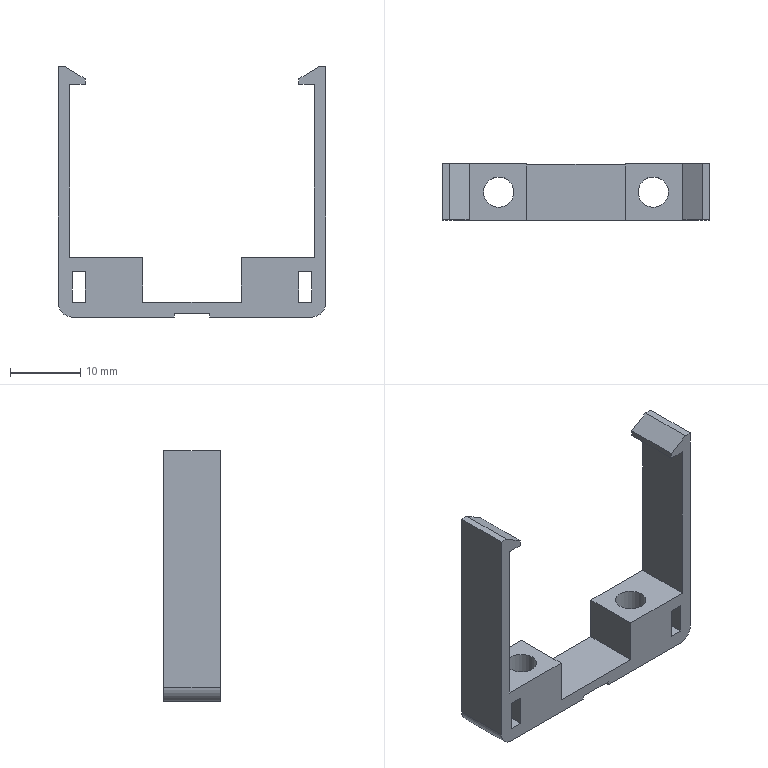Part | NX | 1 solid | 36 faces | box 38 x 8 x 35.6 mm | volume 2200 mm3 | plane 32 | cylinder 4 | commonest cylinder face diameters 4 x2 4.3 x2
STEP:
#1=CARTESIAN_POINT('',(19.85,0.,0.));
#2=VERTEX_POINT('',#1);
#3=CARTESIAN_POINT('',(22.,0.,0.));
#4=DIRECTION('',(0.,0.,1.));
#5=DIRECTION('',(-1.,0.,0.));
#6=AXIS2_PLACEMENT_3D('',#3,#4,#5);
#7=CIRCLE('',#6,2.15);
#8=EDGE_CURVE('',#2,#2,#7,.T.);
#9=ORIENTED_EDGE('',*,*,#8,.T.);
#10=EDGE_LOOP('',(#9));
#11=FACE_BOUND('',#10,.T.);
#12=CARTESIAN_POINT('',(28.,4.,0.));
#13=VERTEX_POINT('',#12);
#14=CARTESIAN_POINT('',(13.5,4.,0.));
#15=VERTEX_POINT('',#14);
#16=CARTESIAN_POINT('',(-8.,4.,0.));
#17=DIRECTION('',(-1.,0.,0.));
#18=VECTOR('',#17,1000.);
#19=LINE('',#16,#18);
#20=EDGE_CURVE('',#13,#15,#19,.T.);
#21=ORIENTED_EDGE('',*,*,#20,.F.);
#22=CARTESIAN_POINT('',(28.,-4.,0.));
#23=VERTEX_POINT('',#22);
#24=CARTESIAN_POINT('',(28.,-4.,0.));
#25=DIRECTION('',(0.,1.,0.));
#26=VECTOR('',#25,1000.);
#27=LINE('',#24,#26);
#28=EDGE_CURVE('',#13,#23,#27,.F.);
#29=ORIENTED_EDGE('',*,*,#28,.T.);
#30=CARTESIAN_POINT('',(13.5,-4.,0.));
#31=VERTEX_POINT('',#30);
#32=CARTESIAN_POINT('',(-8.,-4.,0.));
#33=DIRECTION('',(1.,0.,0.));
#34=VECTOR('',#33,1000.);
#35=LINE('',#32,#34);
#36=EDGE_CURVE('',#31,#23,#35,.T.);
#37=ORIENTED_EDGE('',*,*,#36,.F.);
#38=CARTESIAN_POINT('',(13.5,4.,0.));
#39=DIRECTION('',(0.,-1.,0.));
#40=VECTOR('',#39,1000.);
#41=LINE('',#38,#40);
#42=EDGE_CURVE('',#15,#31,#41,.T.);
#43=ORIENTED_EDGE('',*,*,#42,.F.);
#44=EDGE_LOOP('',(#21,#29,#37,#43));
#45=FACE_BOUND('',#44,.T.);
#46=CARTESIAN_POINT('',(-8.,-4.,0.));
#47=DIRECTION('',(0.,0.,1.));
#48=DIRECTION('',(1.,0.,0.));
#49=AXIS2_PLACEMENT_3D('',#46,#47,#48);
#50=PLANE('',#49);
#51=ADVANCED_FACE('',(#11,#45),#50,.F.);
#52=CARTESIAN_POINT('',(-6.4,-4.,8.5));
#53=VERTEX_POINT('',#52);
#54=CARTESIAN_POINT('',(-6.4,4.,8.5));
#55=VERTEX_POINT('',#54);
#56=CARTESIAN_POINT('',(-6.4,-31.365,8.5));
#57=DIRECTION('',(0.,1.,0.));
#58=VECTOR('',#57,1000.);
#59=LINE('',#56,#58);
#60=EDGE_CURVE('',#53,#55,#59,.T.);
#61=ORIENTED_EDGE('',*,*,#60,.F.);
#62=CARTESIAN_POINT('',(4.,-4.,8.5));
#63=VERTEX_POINT('',#62);
#64=CARTESIAN_POINT('',(-8.,-4.,8.5));
#65=DIRECTION('',(1.,0.,0.));
#66=VECTOR('',#65,1000.);
#67=LINE('',#64,#66);
#68=EDGE_CURVE('',#53,#63,#67,.T.);
#69=ORIENTED_EDGE('',*,*,#68,.T.);
#70=CARTESIAN_POINT('',(4.,4.,8.5));
#71=VERTEX_POINT('',#70);
#72=CARTESIAN_POINT('',(4.,4.,8.5));
#73=DIRECTION('',(0.,-1.,0.));
#74=VECTOR('',#73,1000.);
#75=LINE('',#72,#74);
#76=EDGE_CURVE('',#71,#63,#75,.T.);
#77=ORIENTED_EDGE('',*,*,#76,.F.);
#78=CARTESIAN_POINT('',(-8.,4.,8.5));
#79=DIRECTION('',(-1.,0.,0.));
#80=VECTOR('',#79,1000.);
#81=LINE('',#78,#80);
#82=EDGE_CURVE('',#71,#55,#81,.T.);
#83=ORIENTED_EDGE('',*,*,#82,.T.);
#84=EDGE_LOOP('',(#61,#69,#77,#83));
#85=FACE_BOUND('',#84,.T.);
#86=CARTESIAN_POINT('',(2.15,0.,8.5));
#87=VERTEX_POINT('',#86);
#88=CARTESIAN_POINT('',(0.,0.,8.5));
#89=DIRECTION('',(0.,0.,1.));
#90=DIRECTION('',(1.,0.,0.));
#91=AXIS2_PLACEMENT_3D('',#88,#89,#90);
#92=CIRCLE('',#91,2.15);
#93=EDGE_CURVE('',#87,#87,#92,.T.);
#94=ORIENTED_EDGE('',*,*,#93,.F.);
#95=EDGE_LOOP('',(#94));
#96=FACE_BOUND('',#95,.T.);
#97=CARTESIAN_POINT('',(-8.,-4.,8.5));
#98=DIRECTION('',(0.,0.,1.));
#99=DIRECTION('',(1.,0.,0.));
#100=AXIS2_PLACEMENT_3D('',#97,#98,#99);
#101=PLANE('',#100);
#102=ADVANCED_FACE('',(#85,#96),#101,.T.);
#103=CARTESIAN_POINT('',(28.4,-4.,8.5));
#104=VERTEX_POINT('',#103);
#105=CARTESIAN_POINT('',(28.4,4.,8.5));
#106=VERTEX_POINT('',#105);
#107=CARTESIAN_POINT('',(28.4,-31.365,8.5));
#108=DIRECTION('',(0.,1.,0.));
#109=VECTOR('',#108,1000.);
#110=LINE('',#107,#109);
#111=EDGE_CURVE('',#104,#106,#110,.T.);
#112=ORIENTED_EDGE('',*,*,#111,.T.);
#113=CARTESIAN_POINT('',(18.,4.,8.5));
#114=VERTEX_POINT('',#113);
#115=CARTESIAN_POINT('',(-8.,4.,8.5));
#116=DIRECTION('',(-1.,0.,0.));
#117=VECTOR('',#116,1000.);
#118=LINE('',#115,#117);
#119=EDGE_CURVE('',#106,#114,#118,.T.);
#120=ORIENTED_EDGE('',*,*,#119,.T.);
#121=CARTESIAN_POINT('',(18.,-4.,8.5));
#122=VERTEX_POINT('',#121);
#123=CARTESIAN_POINT('',(18.,4.,8.5));
#124=DIRECTION('',(0.,1.,0.));
#125=VECTOR('',#124,1000.);
#126=LINE('',#123,#125);
#127=EDGE_CURVE('',#122,#114,#126,.T.);
#128=ORIENTED_EDGE('',*,*,#127,.F.);
#129=CARTESIAN_POINT('',(-8.,-4.,8.5));
#130=DIRECTION('',(1.,0.,0.));
#131=VECTOR('',#130,1000.);
#132=LINE('',#129,#131);
#133=EDGE_CURVE('',#122,#104,#132,.T.);
#134=ORIENTED_EDGE('',*,*,#133,.T.);
#135=EDGE_LOOP('',(#112,#120,#128,#134));
#136=FACE_BOUND('',#135,.T.);
#137=CARTESIAN_POINT('',(19.85,0.,8.5));
#138=VERTEX_POINT('',#137);
#139=CARTESIAN_POINT('',(22.,0.,8.5));
#140=DIRECTION('',(0.,0.,1.));
#141=DIRECTION('',(-1.,0.,0.));
#142=AXIS2_PLACEMENT_3D('',#139,#140,#141);
#143=CIRCLE('',#142,2.15);
#144=EDGE_CURVE('',#138,#138,#143,.T.);
#145=ORIENTED_EDGE('',*,*,#144,.F.);
#146=EDGE_LOOP('',(#145));
#147=FACE_BOUND('',#146,.T.);
#148=CARTESIAN_POINT('',(-8.,-4.,8.5));
#149=DIRECTION('',(0.,0.,1.));
#150=DIRECTION('',(1.,0.,0.));
#151=AXIS2_PLACEMENT_3D('',#148,#149,#150);
#152=PLANE('',#151);
#153=ADVANCED_FACE('',(#136,#147),#152,.T.);
#154=CARTESIAN_POINT('',(2.15,0.,0.));
#155=VERTEX_POINT('',#154);
#156=CARTESIAN_POINT('',(0.,0.,0.));
#157=DIRECTION('',(0.,0.,1.));
#158=DIRECTION('',(1.,0.,0.));
#159=AXIS2_PLACEMENT_3D('',#156,#157,#158);
#160=CIRCLE('',#159,2.15);
#161=EDGE_CURVE('',#155,#155,#160,.T.);
#162=ORIENTED_EDGE('',*,*,#161,.T.);
#163=EDGE_LOOP('',(#162));
#164=FACE_BOUND('',#163,.T.);
#165=CARTESIAN_POINT('',(-6.,-4.,0.));
#166=VERTEX_POINT('',#165);
#167=CARTESIAN_POINT('',(8.5,-4.,0.));
#168=VERTEX_POINT('',#167);
#169=CARTESIAN_POINT('',(-8.,-4.,0.));
#170=DIRECTION('',(1.,0.,0.));
#171=VECTOR('',#170,1000.);
#172=LINE('',#169,#171);
#173=EDGE_CURVE('',#166,#168,#172,.T.);
#174=ORIENTED_EDGE('',*,*,#173,.F.);
#175=CARTESIAN_POINT('',(-6.,4.,0.));
#176=VERTEX_POINT('',#175);
#177=CARTESIAN_POINT('',(-6.,-4.,0.));
#178=DIRECTION('',(0.,-1.,0.));
#179=VECTOR('',#178,1000.);
#180=LINE('',#177,#179);
#181=EDGE_CURVE('',#166,#176,#180,.F.);
#182=ORIENTED_EDGE('',*,*,#181,.T.);
#183=CARTESIAN_POINT('',(8.5,4.,0.));
#184=VERTEX_POINT('',#183);
#185=CARTESIAN_POINT('',(-8.,4.,0.));
#186=DIRECTION('',(-1.,0.,0.));
#187=VECTOR('',#186,1000.);
#188=LINE('',#185,#187);
#189=EDGE_CURVE('',#184,#176,#188,.T.);
#190=ORIENTED_EDGE('',*,*,#189,.F.);
#191=CARTESIAN_POINT('',(8.5,4.,0.));
#192=DIRECTION('',(0.,1.,0.));
#193=VECTOR('',#192,1000.);
#194=LINE('',#191,#193);
#195=EDGE_CURVE('',#168,#184,#194,.T.);
#196=ORIENTED_EDGE('',*,*,#195,.F.);
#197=EDGE_LOOP('',(#174,#182,#190,#196));
#198=FACE_BOUND('',#197,.T.);
#199=CARTESIAN_POINT('',(-8.,-4.,0.));
#200=DIRECTION('',(0.,0.,1.));
#201=DIRECTION('',(1.,0.,0.));
#202=AXIS2_PLACEMENT_3D('',#199,#200,#201);
#203=PLANE('',#202);
#204=ADVANCED_FACE('',(#164,#198),#203,.F.);
#205=CARTESIAN_POINT('',(-8.,4.,35.6));
#206=VERTEX_POINT('',#205);
#207=CARTESIAN_POINT('',(-8.,4.,2.));
#208=VERTEX_POINT('',#207);
#209=CARTESIAN_POINT('',(-8.,4.,8.5));
#210=DIRECTION('',(0.,0.,-1.));
#211=VECTOR('',#210,1000.);
#212=LINE('',#209,#211);
#213=EDGE_CURVE('',#206,#208,#212,.T.);
#214=ORIENTED_EDGE('',*,*,#213,.T.);
#215=CARTESIAN_POINT('',(-8.,-4.,2.));
#216=VERTEX_POINT('',#215);
#217=CARTESIAN_POINT('',(-8.,4.,2.));
#218=DIRECTION('',(0.,-1.,0.));
#219=VECTOR('',#218,1000.);
#220=LINE('',#217,#219);
#221=EDGE_CURVE('',#208,#216,#220,.T.);
#222=ORIENTED_EDGE('',*,*,#221,.T.);
#223=CARTESIAN_POINT('',(-8.,-4.,35.6));
#224=VERTEX_POINT('',#223);
#225=CARTESIAN_POINT('',(-8.,-4.,8.5));
#226=DIRECTION('',(0.,0.,-1.));
#227=VECTOR('',#226,1000.);
#228=LINE('',#225,#227);
#229=EDGE_CURVE('',#224,#216,#228,.T.);
#230=ORIENTED_EDGE('',*,*,#229,.F.);
#231=CARTESIAN_POINT('',(-8.,-31.365,35.6));
#232=DIRECTION('',(0.,1.,0.));
#233=VECTOR('',#232,1000.);
#234=LINE('',#231,#233);
#235=EDGE_CURVE('',#224,#206,#234,.T.);
#236=ORIENTED_EDGE('',*,*,#235,.T.);
#237=EDGE_LOOP('',(#214,#222,#230,#236));
#238=FACE_BOUND('',#237,.T.);
#239=CARTESIAN_POINT('',(-8.,4.,8.5));
#240=DIRECTION('',(1.,0.,0.));
#241=DIRECTION('',(0.,0.,-1.));
#242=AXIS2_PLACEMENT_3D('',#239,#240,#241);
#243=PLANE('',#242);
#244=ADVANCED_FACE('',(#238),#243,.F.);
#245=CARTESIAN_POINT('',(28.,-4.,6.5));
#246=VERTEX_POINT('',#245);
#247=CARTESIAN_POINT('',(28.,-4.,2.1));
#248=VERTEX_POINT('',#247);
#249=CARTESIAN_POINT('',(28.,-4.,2.1));
#250=DIRECTION('',(0.,0.,-1.));
#251=VECTOR('',#250,1000.);
#252=LINE('',#249,#251);
#253=EDGE_CURVE('',#246,#248,#252,.T.);
#254=ORIENTED_EDGE('',*,*,#253,.T.);
#255=CARTESIAN_POINT('',(26.15,-4.,2.1));
#256=VERTEX_POINT('',#255);
#257=CARTESIAN_POINT('',(28.,-4.,2.1));
#258=DIRECTION('',(-1.,0.,0.));
#259=VECTOR('',#258,1000.);
#260=LINE('',#257,#259);
#261=EDGE_CURVE('',#248,#256,#260,.T.);
#262=ORIENTED_EDGE('',*,*,#261,.T.);
#263=CARTESIAN_POINT('',(26.15,-4.,6.5));
#264=VERTEX_POINT('',#263);
#265=CARTESIAN_POINT('',(26.15,-4.,2.1));
#266=DIRECTION('',(0.,0.,1.));
#267=VECTOR('',#266,1000.);
#268=LINE('',#265,#267);
#269=EDGE_CURVE('',#256,#264,#268,.T.);
#270=ORIENTED_EDGE('',*,*,#269,.T.);
#271=CARTESIAN_POINT('',(28.,-4.,6.5));
#272=DIRECTION('',(1.,0.,0.));
#273=VECTOR('',#272,1000.);
#274=LINE('',#271,#273);
#275=EDGE_CURVE('',#264,#246,#274,.T.);
#276=ORIENTED_EDGE('',*,*,#275,.T.);
#277=EDGE_LOOP('',(#254,#262,#270,#276));
#278=FACE_BOUND('',#277,.T.);
#279=CARTESIAN_POINT('',(-4.15,-4.,2.1));
#280=VERTEX_POINT('',#279);
#281=CARTESIAN_POINT('',(-6.,-4.,2.1));
#282=VERTEX_POINT('',#281);
#283=CARTESIAN_POINT('',(-6.,-4.,2.1));
#284=DIRECTION('',(-1.,0.,0.));
#285=VECTOR('',#284,1000.);
#286=LINE('',#283,#285);
#287=EDGE_CURVE('',#280,#282,#286,.T.);
#288=ORIENTED_EDGE('',*,*,#287,.T.);
#289=CARTESIAN_POINT('',(-6.,-4.,6.5));
#290=VERTEX_POINT('',#289);
#291=CARTESIAN_POINT('',(-6.,-4.,2.1));
#292=DIRECTION('',(0.,0.,1.));
#293=VECTOR('',#292,1000.);
#294=LINE('',#291,#293);
#295=EDGE_CURVE('',#282,#290,#294,.T.);
#296=ORIENTED_EDGE('',*,*,#295,.T.);
#297=CARTESIAN_POINT('',(-4.15,-4.,6.5));
#298=VERTEX_POINT('',#297);
#299=CARTESIAN_POINT('',(-6.,-4.,6.5));
#300=DIRECTION('',(1.,0.,0.));
#301=VECTOR('',#300,1000.);
#302=LINE('',#299,#301);
#303=EDGE_CURVE('',#290,#298,#302,.T.);
#304=ORIENTED_EDGE('',*,*,#303,.T.);
#305=CARTESIAN_POINT('',(-4.15,-4.,2.1));
#306=DIRECTION('',(0.,0.,-1.));
#307=VECTOR('',#306,1000.);
#308=LINE('',#305,#307);
#309=EDGE_CURVE('',#298,#280,#308,.T.);
#310=ORIENTED_EDGE('',*,*,#309,.T.);
#311=EDGE_LOOP('',(#288,#296,#304,#310));
#312=FACE_BOUND('',#311,.T.);
#313=ORIENTED_EDGE('',*,*,#229,.T.);
#314=CARTESIAN_POINT('',(-6.,-4.,2.));
#315=DIRECTION('',(0.,1.,0.));
#316=DIRECTION('',(-1.,0.,0.));
#317=AXIS2_PLACEMENT_3D('',#314,#315,#316);
#318=CIRCLE('',#317,2.);
#319=EDGE_CURVE('',#216,#166,#318,.F.);
#320=ORIENTED_EDGE('',*,*,#319,.T.);
#321=ORIENTED_EDGE('',*,*,#173,.T.);
#322=CARTESIAN_POINT('',(8.5,-4.,0.5));
#323=VERTEX_POINT('',#322);
#324=CARTESIAN_POINT('',(8.5,-4.,0.5));
#325=DIRECTION('',(0.,0.,-1.));
#326=VECTOR('',#325,1000.);
#327=LINE('',#324,#326);
#328=EDGE_CURVE('',#323,#168,#327,.T.);
#329=ORIENTED_EDGE('',*,*,#328,.F.);
#330=CARTESIAN_POINT('',(13.5,-4.,0.5));
#331=VERTEX_POINT('',#330);
#332=CARTESIAN_POINT('',(13.5,-4.,0.5));
#333=DIRECTION('',(-1.,0.,0.));
#334=VECTOR('',#333,1000.);
#335=LINE('',#332,#334);
#336=EDGE_CURVE('',#331,#323,#335,.T.);
#337=ORIENTED_EDGE('',*,*,#336,.F.);
#338=CARTESIAN_POINT('',(13.5,-4.,0.5));
#339=DIRECTION('',(0.,0.,-1.));
#340=VECTOR('',#339,1000.);
#341=LINE('',#338,#340);
#342=EDGE_CURVE('',#331,#31,#341,.T.);
#343=ORIENTED_EDGE('',*,*,#342,.T.);
#344=ORIENTED_EDGE('',*,*,#36,.T.);
#345=CARTESIAN_POINT('',(30.,-4.,2.));
#346=VERTEX_POINT('',#345);
#347=CARTESIAN_POINT('',(28.,-4.,2.));
#348=DIRECTION('',(0.,1.,0.));
#349=DIRECTION('',(-1.,0.,0.));
#350=AXIS2_PLACEMENT_3D('',#347,#348,#349);
#351=CIRCLE('',#350,2.);
#352=EDGE_CURVE('',#23,#346,#351,.F.);
#353=ORIENTED_EDGE('',*,*,#352,.T.);
#354=CARTESIAN_POINT('',(30.,-4.,35.6));
#355=VERTEX_POINT('',#354);
#356=CARTESIAN_POINT('',(30.,-4.,8.5));
#357=DIRECTION('',(0.,0.,-1.));
#358=VECTOR('',#357,1000.);
#359=LINE('',#356,#358);
#360=EDGE_CURVE('',#355,#346,#359,.T.);
#361=ORIENTED_EDGE('',*,*,#360,.F.);
#362=CARTESIAN_POINT('',(29.,-4.,35.6));
#363=VERTEX_POINT('',#362);
#364=CARTESIAN_POINT('',(30.,-4.,35.6));
#365=DIRECTION('',(-1.,0.,0.));
#366=VECTOR('',#365,1000.);
#367=LINE('',#364,#366);
#368=EDGE_CURVE('',#355,#363,#367,.T.);
#369=ORIENTED_EDGE('',*,*,#368,.T.);
#370=CARTESIAN_POINT('',(26.2,-4.,33.9));
#371=VERTEX_POINT('',#370);
#372=CARTESIAN_POINT('',(26.2,-4.,33.9));
#373=DIRECTION('',(-0.8548,0.,-0.519));
#374=VECTOR('',#373,1000.);
#375=LINE('',#372,#374);
#376=EDGE_CURVE('',#363,#371,#375,.T.);
#377=ORIENTED_EDGE('',*,*,#376,.T.);
#378=CARTESIAN_POINT('',(26.2,-4.,33.1));
#379=VERTEX_POINT('',#378);
#380=CARTESIAN_POINT('',(26.2,-4.,33.1));
#381=DIRECTION('',(0.,0.,-1.));
#382=VECTOR('',#381,1000.);
#383=LINE('',#380,#382);
#384=EDGE_CURVE('',#371,#379,#383,.T.);
#385=ORIENTED_EDGE('',*,*,#384,.T.);
#386=CARTESIAN_POINT('',(28.4,-4.,33.1));
#387=VERTEX_POINT('',#386);
#388=CARTESIAN_POINT('',(28.4,-4.,33.1));
#389=DIRECTION('',(1.,0.,0.));
#390=VECTOR('',#389,1000.);
#391=LINE('',#388,#390);
#392=EDGE_CURVE('',#379,#387,#391,.T.);
#393=ORIENTED_EDGE('',*,*,#392,.T.);
#394=CARTESIAN_POINT('',(28.4,-4.,8.5));
#395=DIRECTION('',(0.,0.,-1.));
#396=VECTOR('',#395,1000.);
#397=LINE('',#394,#396);
#398=EDGE_CURVE('',#387,#104,#397,.T.);
#399=ORIENTED_EDGE('',*,*,#398,.T.);
#400=ORIENTED_EDGE('',*,*,#133,.F.);
#401=CARTESIAN_POINT('',(18.,-4.,2.1));
#402=VERTEX_POINT('',#401);
#403=CARTESIAN_POINT('',(18.,-4.,-16.125));
#404=DIRECTION('',(0.,0.,1.));
#405=VECTOR('',#404,1000.);
#406=LINE('',#403,#405);
#407=EDGE_CURVE('',#402,#122,#406,.T.);
#408=ORIENTED_EDGE('',*,*,#407,.F.);
#409=CARTESIAN_POINT('',(4.,-4.,2.1));
#410=VERTEX_POINT('',#409);
#411=CARTESIAN_POINT('',(4.,-4.,2.1));
#412=DIRECTION('',(-1.,0.,0.));
#413=VECTOR('',#412,1000.);
#414=LINE('',#411,#413);
#415=EDGE_CURVE('',#402,#410,#414,.T.);
#416=ORIENTED_EDGE('',*,*,#415,.T.);
#417=CARTESIAN_POINT('',(4.,-4.,-16.125));
#418=DIRECTION('',(0.,0.,1.));
#419=VECTOR('',#418,1000.);
#420=LINE('',#417,#419);
#421=EDGE_CURVE('',#410,#63,#420,.T.);
#422=ORIENTED_EDGE('',*,*,#421,.T.);
#423=ORIENTED_EDGE('',*,*,#68,.F.);
#424=CARTESIAN_POINT('',(-6.4,-4.,33.1));
#425=VERTEX_POINT('',#424);
#426=CARTESIAN_POINT('',(-6.4,-4.,8.5));
#427=DIRECTION('',(0.,0.,1.));
#428=VECTOR('',#427,1000.);
#429=LINE('',#426,#428);
#430=EDGE_CURVE('',#53,#425,#429,.T.);
#431=ORIENTED_EDGE('',*,*,#430,.T.);
#432=CARTESIAN_POINT('',(-4.2,-4.,33.1));
#433=VERTEX_POINT('',#432);
#434=CARTESIAN_POINT('',(-6.4,-4.,33.1));
#435=DIRECTION('',(1.,0.,0.));
#436=VECTOR('',#435,1000.);
#437=LINE('',#434,#436);
#438=EDGE_CURVE('',#425,#433,#437,.T.);
#439=ORIENTED_EDGE('',*,*,#438,.T.);
#440=CARTESIAN_POINT('',(-4.2,-4.,33.9));
#441=VERTEX_POINT('',#440);
#442=CARTESIAN_POINT('',(-4.2,-4.,33.1));
#443=DIRECTION('',(0.,0.,1.));
#444=VECTOR('',#443,1000.);
#445=LINE('',#442,#444);
#446=EDGE_CURVE('',#433,#441,#445,.T.);
#447=ORIENTED_EDGE('',*,*,#446,.T.);
#448=CARTESIAN_POINT('',(-7.,-4.,35.6));
#449=VERTEX_POINT('',#448);
#450=CARTESIAN_POINT('',(-4.2,-4.,33.9));
#451=DIRECTION('',(-0.8548,0.,0.519));
#452=VECTOR('',#451,1000.);
#453=LINE('',#450,#452);
#454=EDGE_CURVE('',#441,#449,#453,.T.);
#455=ORIENTED_EDGE('',*,*,#454,.T.);
#456=CARTESIAN_POINT('',(-8.,-4.,35.6));
#457=DIRECTION('',(-1.,0.,0.));
#458=VECTOR('',#457,1000.);
#459=LINE('',#456,#458);
#460=EDGE_CURVE('',#449,#224,#459,.T.);
#461=ORIENTED_EDGE('',*,*,#460,.T.);
#462=EDGE_LOOP('',(#313,#320,#321,#329,#337,#343,#344,#353,#361,#369,#377,#385,#393,#399,#400,#408,#416,#422,#423,#431,#439,#447,#455,#461));
#463=FACE_BOUND('',#462,.T.);
#464=CARTESIAN_POINT('',(-8.,-4.,8.5));
#465=DIRECTION('',(0.,1.,0.));
#466=DIRECTION('',(-1.,0.,0.));
#467=AXIS2_PLACEMENT_3D('',#464,#465,#466);
#468=PLANE('',#467);
#469=ADVANCED_FACE('',(#278,#312,#463),#468,.F.);
#470=ORIENTED_EDGE('',*,*,#360,.T.);
#471=CARTESIAN_POINT('',(30.,4.,2.));
#472=VERTEX_POINT('',#471);
#473=CARTESIAN_POINT('',(30.,4.,2.));
#474=DIRECTION('',(0.,1.,0.));
#475=VECTOR('',#474,1000.);
#476=LINE('',#473,#475);
#477=EDGE_CURVE('',#346,#472,#476,.T.);
#478=ORIENTED_EDGE('',*,*,#477,.T.);
#479=CARTESIAN_POINT('',(30.,4.,35.6));
#480=VERTEX_POINT('',#479);
#481=CARTESIAN_POINT('',(30.,4.,8.5));
#482=DIRECTION('',(0.,0.,-1.));
#483=VECTOR('',#482,1000.);
#484=LINE('',#481,#483);
#485=EDGE_CURVE('',#480,#472,#484,.T.);
#486=ORIENTED_EDGE('',*,*,#485,.F.);
#487=CARTESIAN_POINT('',(30.,-31.365,35.6));
#488=DIRECTION('',(0.,1.,0.));
#489=VECTOR('',#488,1000.);
#490=LINE('',#487,#489);
#491=EDGE_CURVE('',#355,#480,#490,.T.);
#492=ORIENTED_EDGE('',*,*,#491,.F.);
#493=EDGE_LOOP('',(#470,#478,#486,#492));
#494=FACE_BOUND('',#493,.T.);
#495=CARTESIAN_POINT('',(30.,4.,8.5));
#496=DIRECTION('',(-1.,0.,0.));
#497=DIRECTION('',(0.,0.,1.));
#498=AXIS2_PLACEMENT_3D('',#495,#496,#497);
#499=PLANE('',#498);
#500=ADVANCED_FACE('',(#494),#499,.F.);
#501=ORIENTED_EDGE('',*,*,#189,.T.);
#502=CARTESIAN_POINT('',(-6.,4.,2.));
#503=DIRECTION('',(0.,-1.,0.));
#504=DIRECTION('',(1.,0.,0.));
#505=AXIS2_PLACEMENT_3D('',#502,#503,#504);
#506=CIRCLE('',#505,2.);
#507=EDGE_CURVE('',#176,#208,#506,.F.);
#508=ORIENTED_EDGE('',*,*,#507,.T.);
#509=ORIENTED_EDGE('',*,*,#213,.F.);
#510=CARTESIAN_POINT('',(-7.,4.,35.6));
#511=VERTEX_POINT('',#510);
#512=CARTESIAN_POINT('',(-8.,4.,35.6));
#513=DIRECTION('',(1.,0.,0.));
#514=VECTOR('',#513,1000.);
#515=LINE('',#512,#514);
#516=EDGE_CURVE('',#206,#511,#515,.T.);
#517=ORIENTED_EDGE('',*,*,#516,.T.);
#518=CARTESIAN_POINT('',(-4.2,4.,33.9));
#519=VERTEX_POINT('',#518);
#520=CARTESIAN_POINT('',(-4.2,4.,33.9));
#521=DIRECTION('',(0.8548,0.,-0.519));
#522=VECTOR('',#521,1000.);
#523=LINE('',#520,#522);
#524=EDGE_CURVE('',#511,#519,#523,.T.);
#525=ORIENTED_EDGE('',*,*,#524,.T.);
#526=CARTESIAN_POINT('',(-4.2,4.,33.1));
#527=VERTEX_POINT('',#526);
#528=CARTESIAN_POINT('',(-4.2,4.,33.1));
#529=DIRECTION('',(0.,0.,-1.));
#530=VECTOR('',#529,1000.);
#531=LINE('',#528,#530);
#532=EDGE_CURVE('',#519,#527,#531,.T.);
#533=ORIENTED_EDGE('',*,*,#532,.T.);
#534=CARTESIAN_POINT('',(-6.4,4.,33.1));
#535=VERTEX_POINT('',#534);
#536=CARTESIAN_POINT('',(-6.4,4.,33.1));
#537=DIRECTION('',(-1.,0.,0.));
#538=VECTOR('',#537,1000.);
#539=LINE('',#536,#538);
#540=EDGE_CURVE('',#527,#535,#539,.T.);
#541=ORIENTED_EDGE('',*,*,#540,.T.);
#542=CARTESIAN_POINT('',(-6.4,4.,8.5));
#543=DIRECTION('',(0.,0.,-1.));
#544=VECTOR('',#543,1000.);
#545=LINE('',#542,#544);
#546=EDGE_CURVE('',#535,#55,#545,.T.);
#547=ORIENTED_EDGE('',*,*,#546,.T.);
#548=ORIENTED_EDGE('',*,*,#82,.F.);
#549=CARTESIAN_POINT('',(4.,4.,2.1));
#550=VERTEX_POINT('',#549);
#551=CARTESIAN_POINT('',(4.,4.,-16.125));
#552=DIRECTION('',(0.,0.,1.));
#553=VECTOR('',#552,1000.);
#554=LINE('',#551,#553);
#555=EDGE_CURVE('',#550,#71,#554,.T.);
#556=ORIENTED_EDGE('',*,*,#555,.F.);
#557=CARTESIAN_POINT('',(18.,4.,2.1));
#558=VERTEX_POINT('',#557);
#559=CARTESIAN_POINT('',(4.,4.,2.1));
#560=DIRECTION('',(1.,0.,0.));
#561=VECTOR('',#560,1000.);
#562=LINE('',#559,#561);
#563=EDGE_CURVE('',#550,#558,#562,.T.);
#564=ORIENTED_EDGE('',*,*,#563,.T.);
#565=CARTESIAN_POINT('',(18.,4.,-16.125));
#566=DIRECTION('',(0.,0.,1.));
#567=VECTOR('',#566,1000.);
#568=LINE('',#565,#567);
#569=EDGE_CURVE('',#558,#114,#568,.T.);
#570=ORIENTED_EDGE('',*,*,#569,.T.);
#571=ORIENTED_EDGE('',*,*,#119,.F.);
#572=CARTESIAN_POINT('',(28.4,4.,33.1));
#573=VERTEX_POINT('',#572);
#574=CARTESIAN_POINT('',(28.4,4.,8.5));
#575=DIRECTION('',(0.,0.,1.));
#576=VECTOR('',#575,1000.);
#577=LINE('',#574,#576);
#578=EDGE_CURVE('',#106,#573,#577,.T.);
#579=ORIENTED_EDGE('',*,*,#578,.T.);
#580=CARTESIAN_POINT('',(26.2,4.,33.1));
#581=VERTEX_POINT('',#580);
#582=CARTESIAN_POINT('',(28.4,4.,33.1));
#583=DIRECTION('',(-1.,0.,0.));
#584=VECTOR('',#583,1000.);
#585=LINE('',#582,#584);
#586=EDGE_CURVE('',#573,#581,#585,.T.);
#587=ORIENTED_EDGE('',*,*,#586,.T.);
#588=CARTESIAN_POINT('',(26.2,4.,33.9));
#589=VERTEX_POINT('',#588);
#590=CARTESIAN_POINT('',(26.2,4.,33.1));
#591=DIRECTION('',(0.,0.,1.));
#592=VECTOR('',#591,1000.);
#593=LINE('',#590,#592);
#594=EDGE_CURVE('',#581,#589,#593,.T.);
#595=ORIENTED_EDGE('',*,*,#594,.T.);
#596=CARTESIAN_POINT('',(29.,4.,35.6));
#597=VERTEX_POINT('',#596);
#598=CARTESIAN_POINT('',(26.2,4.,33.9));
#599=DIRECTION('',(0.8548,0.,0.519));
#600=VECTOR('',#599,1000.);
#601=LINE('',#598,#600);
#602=EDGE_CURVE('',#589,#597,#601,.T.);
#603=ORIENTED_EDGE('',*,*,#602,.T.);
#604=CARTESIAN_POINT('',(30.,4.,35.6));
#605=DIRECTION('',(1.,0.,0.));
#606=VECTOR('',#605,1000.);
#607=LINE('',#604,#606);
#608=EDGE_CURVE('',#597,#480,#607,.T.);
#609=ORIENTED_EDGE('',*,*,#608,.T.);
#610=ORIENTED_EDGE('',*,*,#485,.T.);
#611=CARTESIAN_POINT('',(28.,4.,2.));
#612=DIRECTION('',(0.,-1.,0.));
#613=DIRECTION('',(1.,0.,0.));
#614=AXIS2_PLACEMENT_3D('',#611,#612,#613);
#615=CIRCLE('',#614,2.);
#616=EDGE_CURVE('',#472,#13,#615,.F.);
#617=ORIENTED_EDGE('',*,*,#616,.T.);
#618=ORIENTED_EDGE('',*,*,#20,.T.);
#619=CARTESIAN_POINT('',(13.5,4.,0.5));
#620=VERTEX_POINT('',#619);
#621=CARTESIAN_POINT('',(13.5,4.,0.5));
#622=DIRECTION('',(0.,0.,-1.));
#623=VECTOR('',#622,1000.);
#624=LINE('',#621,#623);
#625=EDGE_CURVE('',#620,#15,#624,.T.);
#626=ORIENTED_EDGE('',*,*,#625,.F.);
#627=CARTESIAN_POINT('',(8.5,4.,0.5));
#628=VERTEX_POINT('',#627);
#629=CARTESIAN_POINT('',(13.5,4.,0.5));
#630=DIRECTION('',(1.,0.,0.));
#631=VECTOR('',#630,1000.);
#632=LINE('',#629,#631);
#633=EDGE_CURVE('',#628,#620,#632,.T.);
#634=ORIENTED_EDGE('',*,*,#633,.F.);
#635=CARTESIAN_POINT('',(8.5,4.,0.5));
#636=DIRECTION('',(0.,0.,-1.));
#637=VECTOR('',#636,1000.);
#638=LINE('',#635,#637);
#639=EDGE_CURVE('',#628,#184,#638,.T.);
#640=ORIENTED_EDGE('',*,*,#639,.T.);
#641=EDGE_LOOP('',(#501,#508,#509,#517,#525,#533,#541,#547,#548,#556,#564,#570,#571,#579,#587,#595,#603,#609,#610,#617,#618,#626,#634,#640));
#642=FACE_BOUND('',#641,.T.);
#643=CARTESIAN_POINT('',(26.15,4.,2.1));
#644=VERTEX_POINT('',#643);
#645=CARTESIAN_POINT('',(26.15,4.,6.5));
#646=VERTEX_POINT('',#645);
#647=CARTESIAN_POINT('',(26.15,4.,2.1));
#648=DIRECTION('',(0.,0.,1.));
#649=VECTOR('',#648,1000.);
#650=LINE('',#647,#649);
#651=EDGE_CURVE('',#644,#646,#650,.T.);
#652=ORIENTED_EDGE('',*,*,#651,.F.);
#653=CARTESIAN_POINT('',(28.,4.,2.1));
#654=VERTEX_POINT('',#653);
#655=CARTESIAN_POINT('',(28.,4.,2.1));
#656=DIRECTION('',(-1.,0.,0.));
#657=VECTOR('',#656,1000.);
#658=LINE('',#655,#657);
#659=EDGE_CURVE('',#654,#644,#658,.T.);
#660=ORIENTED_EDGE('',*,*,#659,.F.);
#661=CARTESIAN_POINT('',(28.,4.,6.5));
#662=VERTEX_POINT('',#661);
#663=CARTESIAN_POINT('',(28.,4.,2.1));
#664=DIRECTION('',(0.,0.,-1.));
#665=VECTOR('',#664,1000.);
#666=LINE('',#663,#665);
#667=EDGE_CURVE('',#662,#654,#666,.T.);
#668=ORIENTED_EDGE('',*,*,#667,.F.);
#669=CARTESIAN_POINT('',(28.,4.,6.5));
#670=DIRECTION('',(1.,0.,0.));
#671=VECTOR('',#670,1000.);
#672=LINE('',#669,#671);
#673=EDGE_CURVE('',#646,#662,#672,.T.);
#674=ORIENTED_EDGE('',*,*,#673,.F.);
#675=EDGE_LOOP('',(#652,#660,#668,#674));
#676=FACE_BOUND('',#675,.T.);
#677=CARTESIAN_POINT('',(-6.,4.,6.5));
#678=VERTEX_POINT('',#677);
#679=CARTESIAN_POINT('',(-4.15,4.,6.5));
#680=VERTEX_POINT('',#679);
#681=CARTESIAN_POINT('',(-6.,4.,6.5));
#682=DIRECTION('',(1.,0.,0.));
#683=VECTOR('',#682,1000.);
#684=LINE('',#681,#683);
#685=EDGE_CURVE('',#678,#680,#684,.T.);
#686=ORIENTED_EDGE('',*,*,#685,.F.);
#687=CARTESIAN_POINT('',(-6.,4.,2.1));
#688=VERTEX_POINT('',#687);
#689=CARTESIAN_POINT('',(-6.,4.,2.1));
#690=DIRECTION('',(0.,0.,1.));
#691=VECTOR('',#690,1000.);
#692=LINE('',#689,#691);
#693=EDGE_CURVE('',#688,#678,#692,.T.);
#694=ORIENTED_EDGE('',*,*,#693,.F.);
#695=CARTESIAN_POINT('',(-4.15,4.,2.1));
#696=VERTEX_POINT('',#695);
#697=CARTESIAN_POINT('',(-6.,4.,2.1));
#698=DIRECTION('',(-1.,0.,0.));
#699=VECTOR('',#698,1000.);
#700=LINE('',#697,#699);
#701=EDGE_CURVE('',#696,#688,#700,.T.);
#702=ORIENTED_EDGE('',*,*,#701,.F.);
#703=CARTESIAN_POINT('',(-4.15,4.,2.1));
#704=DIRECTION('',(0.,0.,-1.));
#705=VECTOR('',#704,1000.);
#706=LINE('',#703,#705);
#707=EDGE_CURVE('',#680,#696,#706,.T.);
#708=ORIENTED_EDGE('',*,*,#707,.F.);
#709=EDGE_LOOP('',(#686,#694,#702,#708));
#710=FACE_BOUND('',#709,.T.);
#711=CARTESIAN_POINT('',(-8.,4.,8.5));
#712=DIRECTION('',(0.,-1.,0.));
#713=DIRECTION('',(1.,0.,0.));
#714=AXIS2_PLACEMENT_3D('',#711,#712,#713);
#715=PLANE('',#714);
#716=ADVANCED_FACE('',(#642,#676,#710),#715,.F.);
#717=ORIENTED_EDGE('',*,*,#93,.T.);
#718=EDGE_LOOP('',(#717));
#719=FACE_BOUND('',#718,.T.);
#720=ORIENTED_EDGE('',*,*,#161,.F.);
#721=EDGE_LOOP('',(#720));
#722=FACE_BOUND('',#721,.T.);
#723=CARTESIAN_POINT('',(0.,0.,8.5));
#724=DIRECTION('',(0.,0.,-1.));
#725=DIRECTION('',(-1.,0.,0.));
#726=AXIS2_PLACEMENT_3D('',#723,#724,#725);
#727=CYLINDRICAL_SURFACE('',#726,2.15);
#728=ADVANCED_FACE('',(#719,#722),#727,.F.);
#729=ORIENTED_EDGE('',*,*,#144,.T.);
#730=EDGE_LOOP('',(#729));
#731=FACE_BOUND('',#730,.T.);
#732=ORIENTED_EDGE('',*,*,#8,.F.);
#733=EDGE_LOOP('',(#732));
#734=FACE_BOUND('',#733,.T.);
#735=CARTESIAN_POINT('',(22.,0.,8.5));
#736=DIRECTION('',(0.,0.,-1.));
#737=DIRECTION('',(-1.,0.,0.));
#738=AXIS2_PLACEMENT_3D('',#735,#736,#737);
#739=CYLINDRICAL_SURFACE('',#738,2.15);
#740=ADVANCED_FACE('',(#731,#734),#739,.F.);
#741=CARTESIAN_POINT('',(4.,4.,2.1));
#742=DIRECTION('',(0.,1.,0.));
#743=VECTOR('',#742,1000.);
#744=LINE('',#741,#743);
#745=EDGE_CURVE('',#410,#550,#744,.T.);
#746=ORIENTED_EDGE('',*,*,#745,.T.);
#747=ORIENTED_EDGE('',*,*,#555,.T.);
#748=ORIENTED_EDGE('',*,*,#76,.T.);
#749=ORIENTED_EDGE('',*,*,#421,.F.);
#750=EDGE_LOOP('',(#746,#747,#748,#749));
#751=FACE_BOUND('',#750,.T.);
#752=CARTESIAN_POINT('',(4.,4.,-16.125));
#753=DIRECTION('',(-1.,0.,0.));
#754=DIRECTION('',(0.,-1.,0.));
#755=AXIS2_PLACEMENT_3D('',#752,#753,#754);
#756=PLANE('',#755);
#757=ADVANCED_FACE('',(#751),#756,.F.);
#758=CARTESIAN_POINT('',(18.,4.,2.1));
#759=DIRECTION('',(0.,-1.,0.));
#760=VECTOR('',#759,1000.);
#761=LINE('',#758,#760);
#762=EDGE_CURVE('',#558,#402,#761,.T.);
#763=ORIENTED_EDGE('',*,*,#762,.T.);
#764=ORIENTED_EDGE('',*,*,#407,.T.);
#765=ORIENTED_EDGE('',*,*,#127,.T.);
#766=ORIENTED_EDGE('',*,*,#569,.F.);
#767=EDGE_LOOP('',(#763,#764,#765,#766));
#768=FACE_BOUND('',#767,.T.);
#769=CARTESIAN_POINT('',(18.,4.,-16.125));
#770=DIRECTION('',(1.,0.,0.));
#771=DIRECTION('',(0.,0.,-1.));
#772=AXIS2_PLACEMENT_3D('',#769,#770,#771);
#773=PLANE('',#772);
#774=ADVANCED_FACE('',(#768),#773,.F.);
#775=ORIENTED_EDGE('',*,*,#745,.F.);
#776=ORIENTED_EDGE('',*,*,#415,.F.);
#777=ORIENTED_EDGE('',*,*,#762,.F.);
#778=ORIENTED_EDGE('',*,*,#563,.F.);
#779=EDGE_LOOP('',(#775,#776,#777,#778));
#780=FACE_BOUND('',#779,.T.);
#781=CARTESIAN_POINT('',(-8.,-4.,2.1));
#782=DIRECTION('',(0.,0.,1.));
#783=DIRECTION('',(1.,0.,0.));
#784=AXIS2_PLACEMENT_3D('',#781,#782,#783);
#785=PLANE('',#784);
#786=ADVANCED_FACE('',(#780),#785,.T.);
#787=ORIENTED_EDGE('',*,*,#430,.F.);
#788=ORIENTED_EDGE('',*,*,#60,.T.);
#789=ORIENTED_EDGE('',*,*,#546,.F.);
#790=CARTESIAN_POINT('',(-6.4,-31.365,33.1));
#791=DIRECTION('',(0.,1.,0.));
#792=VECTOR('',#791,1000.);
#793=LINE('',#790,#792);
#794=EDGE_CURVE('',#425,#535,#793,.T.);
#795=ORIENTED_EDGE('',*,*,#794,.F.);
#796=EDGE_LOOP('',(#787,#788,#789,#795));
#797=FACE_BOUND('',#796,.T.);
#798=CARTESIAN_POINT('',(-6.4,-31.365,8.5));
#799=DIRECTION('',(1.,0.,0.));
#800=DIRECTION('',(0.,1.,0.));
#801=AXIS2_PLACEMENT_3D('',#798,#799,#800);
#802=PLANE('',#801);
#803=ADVANCED_FACE('',(#797),#802,.T.);
#804=ORIENTED_EDGE('',*,*,#438,.F.);
#805=ORIENTED_EDGE('',*,*,#794,.T.);
#806=ORIENTED_EDGE('',*,*,#540,.F.);
#807=CARTESIAN_POINT('',(-4.2,-31.365,33.1));
#808=DIRECTION('',(0.,1.,0.));
#809=VECTOR('',#808,1000.);
#810=LINE('',#807,#809);
#811=EDGE_CURVE('',#433,#527,#810,.T.);
#812=ORIENTED_EDGE('',*,*,#811,.F.);
#813=EDGE_LOOP('',(#804,#805,#806,#812));
#814=FACE_BOUND('',#813,.T.);
#815=CARTESIAN_POINT('',(-6.4,-31.365,33.1));
#816=DIRECTION('',(0.,0.,-1.));
#817=DIRECTION('',(-1.,0.,0.));
#818=AXIS2_PLACEMENT_3D('',#815,#816,#817);
#819=PLANE('',#818);
#820=ADVANCED_FACE('',(#814),#819,.T.);
#821=ORIENTED_EDGE('',*,*,#446,.F.);
#822=ORIENTED_EDGE('',*,*,#811,.T.);
#823=ORIENTED_EDGE('',*,*,#532,.F.);
#824=CARTESIAN_POINT('',(-4.2,-31.365,33.9));
#825=DIRECTION('',(0.,1.,0.));
#826=VECTOR('',#825,1000.);
#827=LINE('',#824,#826);
#828=EDGE_CURVE('',#441,#519,#827,.T.);
#829=ORIENTED_EDGE('',*,*,#828,.F.);
#830=EDGE_LOOP('',(#821,#822,#823,#829));
#831=FACE_BOUND('',#830,.T.);
#832=CARTESIAN_POINT('',(-4.2,-31.365,33.1));
#833=DIRECTION('',(1.,0.,0.));
#834=DIRECTION('',(0.,1.,0.));
#835=AXIS2_PLACEMENT_3D('',#832,#833,#834);
#836=PLANE('',#835);
#837=ADVANCED_FACE('',(#831),#836,.T.);
#838=ORIENTED_EDGE('',*,*,#454,.F.);
#839=ORIENTED_EDGE('',*,*,#828,.T.);
#840=ORIENTED_EDGE('',*,*,#524,.F.);
#841=CARTESIAN_POINT('',(-7.,-31.365,35.6));
#842=DIRECTION('',(0.,1.,0.));
#843=VECTOR('',#842,1000.);
#844=LINE('',#841,#843);
#845=EDGE_CURVE('',#449,#511,#844,.T.);
#846=ORIENTED_EDGE('',*,*,#845,.F.);
#847=EDGE_LOOP('',(#838,#839,#840,#846));
#848=FACE_BOUND('',#847,.T.);
#849=CARTESIAN_POINT('',(-4.2,-31.365,33.9));
#850=DIRECTION('',(0.519,0.,0.8548));
#851=DIRECTION('',(0.8548,0.,-0.519));
#852=AXIS2_PLACEMENT_3D('',#849,#850,#851);
#853=PLANE('',#852);
#854=ADVANCED_FACE('',(#848),#853,.T.);
#855=ORIENTED_EDGE('',*,*,#460,.F.);
#856=ORIENTED_EDGE('',*,*,#845,.T.);
#857=ORIENTED_EDGE('',*,*,#516,.F.);
#858=ORIENTED_EDGE('',*,*,#235,.F.);
#859=EDGE_LOOP('',(#855,#856,#857,#858));
#860=FACE_BOUND('',#859,.T.);
#861=CARTESIAN_POINT('',(-8.,-31.365,35.6));
#862=DIRECTION('',(0.,0.,1.));
#863=DIRECTION('',(1.,0.,0.));
#864=AXIS2_PLACEMENT_3D('',#861,#862,#863);
#865=PLANE('',#864);
#866=ADVANCED_FACE('',(#860),#865,.T.);
#867=ORIENTED_EDGE('',*,*,#384,.F.);
#868=CARTESIAN_POINT('',(26.2,-31.365,33.9));
#869=DIRECTION('',(0.,1.,0.));
#870=VECTOR('',#869,1000.);
#871=LINE('',#868,#870);
#872=EDGE_CURVE('',#371,#589,#871,.T.);
#873=ORIENTED_EDGE('',*,*,#872,.T.);
#874=ORIENTED_EDGE('',*,*,#594,.F.);
#875=CARTESIAN_POINT('',(26.2,-31.365,33.1));
#876=DIRECTION('',(0.,1.,0.));
#877=VECTOR('',#876,1000.);
#878=LINE('',#875,#877);
#879=EDGE_CURVE('',#379,#581,#878,.T.);
#880=ORIENTED_EDGE('',*,*,#879,.F.);
#881=EDGE_LOOP('',(#867,#873,#874,#880));
#882=FACE_BOUND('',#881,.T.);
#883=CARTESIAN_POINT('',(26.2,-31.365,33.1));
#884=DIRECTION('',(-1.,0.,0.));
#885=DIRECTION('',(0.,-1.,0.));
#886=AXIS2_PLACEMENT_3D('',#883,#884,#885);
#887=PLANE('',#886);
#888=ADVANCED_FACE('',(#882),#887,.T.);
#889=ORIENTED_EDGE('',*,*,#392,.F.);
#890=ORIENTED_EDGE('',*,*,#879,.T.);
#891=ORIENTED_EDGE('',*,*,#586,.F.);
#892=CARTESIAN_POINT('',(28.4,-31.365,33.1));
#893=DIRECTION('',(0.,1.,0.));
#894=VECTOR('',#893,1000.);
#895=LINE('',#892,#894);
#896=EDGE_CURVE('',#387,#573,#895,.T.);
#897=ORIENTED_EDGE('',*,*,#896,.F.);
#898=EDGE_LOOP('',(#889,#890,#891,#897));
#899=FACE_BOUND('',#898,.T.);
#900=CARTESIAN_POINT('',(28.4,-31.365,33.1));
#901=DIRECTION('',(0.,0.,-1.));
#902=DIRECTION('',(-1.,0.,0.));
#903=AXIS2_PLACEMENT_3D('',#900,#901,#902);
#904=PLANE('',#903);
#905=ADVANCED_FACE('',(#899),#904,.T.);
#906=ORIENTED_EDGE('',*,*,#398,.F.);
#907=ORIENTED_EDGE('',*,*,#896,.T.);
#908=ORIENTED_EDGE('',*,*,#578,.F.);
#909=ORIENTED_EDGE('',*,*,#111,.F.);
#910=EDGE_LOOP('',(#906,#907,#908,#909));
#911=FACE_BOUND('',#910,.T.);
#912=CARTESIAN_POINT('',(28.4,-31.365,8.5));
#913=DIRECTION('',(-1.,0.,0.));
#914=DIRECTION('',(0.,-1.,0.));
#915=AXIS2_PLACEMENT_3D('',#912,#913,#914);
#916=PLANE('',#915);
#917=ADVANCED_FACE('',(#911),#916,.T.);
#918=ORIENTED_EDGE('',*,*,#368,.F.);
#919=ORIENTED_EDGE('',*,*,#491,.T.);
#920=ORIENTED_EDGE('',*,*,#608,.F.);
#921=CARTESIAN_POINT('',(29.,-31.365,35.6));
#922=DIRECTION('',(0.,1.,0.));
#923=VECTOR('',#922,1000.);
#924=LINE('',#921,#923);
#925=EDGE_CURVE('',#363,#597,#924,.T.);
#926=ORIENTED_EDGE('',*,*,#925,.F.);
#927=EDGE_LOOP('',(#918,#919,#920,#926));
#928=FACE_BOUND('',#927,.T.);
#929=CARTESIAN_POINT('',(30.,-31.365,35.6));
#930=DIRECTION('',(0.,0.,1.));
#931=DIRECTION('',(1.,0.,0.));
#932=AXIS2_PLACEMENT_3D('',#929,#930,#931);
#933=PLANE('',#932);
#934=ADVANCED_FACE('',(#928),#933,.T.);
#935=ORIENTED_EDGE('',*,*,#376,.F.);
#936=ORIENTED_EDGE('',*,*,#925,.T.);
#937=ORIENTED_EDGE('',*,*,#602,.F.);
#938=ORIENTED_EDGE('',*,*,#872,.F.);
#939=EDGE_LOOP('',(#935,#936,#937,#938));
#940=FACE_BOUND('',#939,.T.);
#941=CARTESIAN_POINT('',(26.2,-31.365,33.9));
#942=DIRECTION('',(-0.519,0.,0.8548));
#943=DIRECTION('',(0.8548,0.,0.519));
#944=AXIS2_PLACEMENT_3D('',#941,#942,#943);
#945=PLANE('',#944);
#946=ADVANCED_FACE('',(#940),#945,.T.);
#947=ORIENTED_EDGE('',*,*,#693,.T.);
#948=CARTESIAN_POINT('',(-6.,-4.,6.5));
#949=DIRECTION('',(0.,1.,0.));
#950=VECTOR('',#949,1000.);
#951=LINE('',#948,#950);
#952=EDGE_CURVE('',#290,#678,#951,.T.);
#953=ORIENTED_EDGE('',*,*,#952,.F.);
#954=ORIENTED_EDGE('',*,*,#295,.F.);
#955=CARTESIAN_POINT('',(-6.,-4.,2.1));
#956=DIRECTION('',(0.,1.,0.));
#957=VECTOR('',#956,1000.);
#958=LINE('',#955,#957);
#959=EDGE_CURVE('',#282,#688,#958,.T.);
#960=ORIENTED_EDGE('',*,*,#959,.T.);
#961=EDGE_LOOP('',(#947,#953,#954,#960));
#962=FACE_BOUND('',#961,.T.);
#963=CARTESIAN_POINT('',(-6.,-4.,2.1));
#964=DIRECTION('',(-1.,0.,0.));
#965=DIRECTION('',(0.,-1.,0.));
#966=AXIS2_PLACEMENT_3D('',#963,#964,#965);
#967=PLANE('',#966);
#968=ADVANCED_FACE('',(#962),#967,.F.);
#969=ORIENTED_EDGE('',*,*,#701,.T.);
#970=ORIENTED_EDGE('',*,*,#959,.F.);
#971=ORIENTED_EDGE('',*,*,#287,.F.);
#972=CARTESIAN_POINT('',(-4.15,-4.,2.1));
#973=DIRECTION('',(0.,1.,0.));
#974=VECTOR('',#973,1000.);
#975=LINE('',#972,#974);
#976=EDGE_CURVE('',#280,#696,#975,.T.);
#977=ORIENTED_EDGE('',*,*,#976,.T.);
#978=EDGE_LOOP('',(#969,#970,#971,#977));
#979=FACE_BOUND('',#978,.T.);
#980=CARTESIAN_POINT('',(-6.,-4.,2.1));
#981=DIRECTION('',(0.,0.,-1.));
#982=DIRECTION('',(-1.,0.,0.));
#983=AXIS2_PLACEMENT_3D('',#980,#981,#982);
#984=PLANE('',#983);
#985=ADVANCED_FACE('',(#979),#984,.F.);
#986=ORIENTED_EDGE('',*,*,#707,.T.);
#987=ORIENTED_EDGE('',*,*,#976,.F.);
#988=ORIENTED_EDGE('',*,*,#309,.F.);
#989=CARTESIAN_POINT('',(-4.15,-4.,6.5));
#990=DIRECTION('',(0.,1.,0.));
#991=VECTOR('',#990,1000.);
#992=LINE('',#989,#991);
#993=EDGE_CURVE('',#298,#680,#992,.T.);
#994=ORIENTED_EDGE('',*,*,#993,.T.);
#995=EDGE_LOOP('',(#986,#987,#988,#994));
#996=FACE_BOUND('',#995,.T.);
#997=CARTESIAN_POINT('',(-4.15,-4.,2.1));
#998=DIRECTION('',(1.,0.,0.));
#999=DIRECTION('',(0.,1.,0.));
#1000=AXIS2_PLACEMENT_3D('',#997,#998,#999);
#1001=PLANE('',#1000);
#1002=ADVANCED_FACE('',(#996),#1001,.F.);
#1003=ORIENTED_EDGE('',*,*,#685,.T.);
#1004=ORIENTED_EDGE('',*,*,#993,.F.);
#1005=ORIENTED_EDGE('',*,*,#303,.F.);
#1006=ORIENTED_EDGE('',*,*,#952,.T.);
#1007=EDGE_LOOP('',(#1003,#1004,#1005,#1006));
#1008=FACE_BOUND('',#1007,.T.);
#1009=CARTESIAN_POINT('',(-6.,-4.,6.5));
#1010=DIRECTION('',(0.,0.,1.));
#1011=DIRECTION('',(1.,0.,0.));
#1012=AXIS2_PLACEMENT_3D('',#1009,#1010,#1011);
#1013=PLANE('',#1012);
#1014=ADVANCED_FACE('',(#1008),#1013,.F.);
#1015=ORIENTED_EDGE('',*,*,#659,.T.);
#1016=CARTESIAN_POINT('',(26.15,-4.,2.1));
#1017=DIRECTION('',(0.,1.,0.));
#1018=VECTOR('',#1017,1000.);
#1019=LINE('',#1016,#1018);
#1020=EDGE_CURVE('',#256,#644,#1019,.T.);
#1021=ORIENTED_EDGE('',*,*,#1020,.F.);
#1022=ORIENTED_EDGE('',*,*,#261,.F.);
#1023=CARTESIAN_POINT('',(28.,-4.,2.1));
#1024=DIRECTION('',(0.,1.,0.));
#1025=VECTOR('',#1024,1000.);
#1026=LINE('',#1023,#1025);
#1027=EDGE_CURVE('',#248,#654,#1026,.T.);
#1028=ORIENTED_EDGE('',*,*,#1027,.T.);
#1029=EDGE_LOOP('',(#1015,#1021,#1022,#1028));
#1030=FACE_BOUND('',#1029,.T.);
#1031=CARTESIAN_POINT('',(28.,-4.,2.1));
#1032=DIRECTION('',(0.,0.,-1.));
#1033=DIRECTION('',(-1.,0.,0.));
#1034=AXIS2_PLACEMENT_3D('',#1031,#1032,#1033);
#1035=PLANE('',#1034);
#1036=ADVANCED_FACE('',(#1030),#1035,.F.);
#1037=ORIENTED_EDGE('',*,*,#667,.T.);
#1038=ORIENTED_EDGE('',*,*,#1027,.F.);
#1039=ORIENTED_EDGE('',*,*,#253,.F.);
#1040=CARTESIAN_POINT('',(28.,-4.,6.5));
#1041=DIRECTION('',(0.,1.,0.));
#1042=VECTOR('',#1041,1000.);
#1043=LINE('',#1040,#1042);
#1044=EDGE_CURVE('',#246,#662,#1043,.T.);
#1045=ORIENTED_EDGE('',*,*,#1044,.T.);
#1046=EDGE_LOOP('',(#1037,#1038,#1039,#1045));
#1047=FACE_BOUND('',#1046,.T.);
#1048=CARTESIAN_POINT('',(28.,-4.,2.1));
#1049=DIRECTION('',(1.,0.,0.));
#1050=DIRECTION('',(0.,1.,0.));
#1051=AXIS2_PLACEMENT_3D('',#1048,#1049,#1050);
#1052=PLANE('',#1051);
#1053=ADVANCED_FACE('',(#1047),#1052,.F.);
#1054=ORIENTED_EDGE('',*,*,#673,.T.);
#1055=ORIENTED_EDGE('',*,*,#1044,.F.);
#1056=ORIENTED_EDGE('',*,*,#275,.F.);
#1057=CARTESIAN_POINT('',(26.15,-4.,6.5));
#1058=DIRECTION('',(0.,1.,0.));
#1059=VECTOR('',#1058,1000.);
#1060=LINE('',#1057,#1059);
#1061=EDGE_CURVE('',#264,#646,#1060,.T.);
#1062=ORIENTED_EDGE('',*,*,#1061,.T.);
#1063=EDGE_LOOP('',(#1054,#1055,#1056,#1062));
#1064=FACE_BOUND('',#1063,.T.);
#1065=CARTESIAN_POINT('',(28.,-4.,6.5));
#1066=DIRECTION('',(0.,0.,1.));
#1067=DIRECTION('',(1.,0.,0.));
#1068=AXIS2_PLACEMENT_3D('',#1065,#1066,#1067);
#1069=PLANE('',#1068);
#1070=ADVANCED_FACE('',(#1064),#1069,.F.);
#1071=ORIENTED_EDGE('',*,*,#651,.T.);
#1072=ORIENTED_EDGE('',*,*,#1061,.F.);
#1073=ORIENTED_EDGE('',*,*,#269,.F.);
#1074=ORIENTED_EDGE('',*,*,#1020,.T.);
#1075=EDGE_LOOP('',(#1071,#1072,#1073,#1074));
#1076=FACE_BOUND('',#1075,.T.);
#1077=CARTESIAN_POINT('',(26.15,-4.,2.1));
#1078=DIRECTION('',(-1.,0.,0.));
#1079=DIRECTION('',(0.,-1.,0.));
#1080=AXIS2_PLACEMENT_3D('',#1077,#1078,#1079);
#1081=PLANE('',#1080);
#1082=ADVANCED_FACE('',(#1076),#1081,.F.);
#1083=ORIENTED_EDGE('',*,*,#42,.T.);
#1084=ORIENTED_EDGE('',*,*,#342,.F.);
#1085=CARTESIAN_POINT('',(13.5,4.,0.5));
#1086=DIRECTION('',(0.,-1.,0.));
#1087=VECTOR('',#1086,1000.);
#1088=LINE('',#1085,#1087);
#1089=EDGE_CURVE('',#620,#331,#1088,.T.);
#1090=ORIENTED_EDGE('',*,*,#1089,.F.);
#1091=ORIENTED_EDGE('',*,*,#625,.T.);
#1092=EDGE_LOOP('',(#1083,#1084,#1090,#1091));
#1093=FACE_BOUND('',#1092,.T.);
#1094=CARTESIAN_POINT('',(13.5,4.,0.5));
#1095=DIRECTION('',(1.,0.,0.));
#1096=DIRECTION('',(0.,1.,0.));
#1097=AXIS2_PLACEMENT_3D('',#1094,#1095,#1096);
#1098=PLANE('',#1097);
#1099=ADVANCED_FACE('',(#1093),#1098,.F.);
#1100=ORIENTED_EDGE('',*,*,#195,.T.);
#1101=ORIENTED_EDGE('',*,*,#639,.F.);
#1102=CARTESIAN_POINT('',(8.5,4.,0.5));
#1103=DIRECTION('',(0.,1.,0.));
#1104=VECTOR('',#1103,1000.);
#1105=LINE('',#1102,#1104);
#1106=EDGE_CURVE('',#323,#628,#1105,.T.);
#1107=ORIENTED_EDGE('',*,*,#1106,.F.);
#1108=ORIENTED_EDGE('',*,*,#328,.T.);
#1109=EDGE_LOOP('',(#1100,#1101,#1107,#1108));
#1110=FACE_BOUND('',#1109,.T.);
#1111=CARTESIAN_POINT('',(8.5,4.,0.5));
#1112=DIRECTION('',(-1.,0.,0.));
#1113=DIRECTION('',(0.,0.,1.));
#1114=AXIS2_PLACEMENT_3D('',#1111,#1112,#1113);
#1115=PLANE('',#1114);
#1116=ADVANCED_FACE('',(#1110),#1115,.F.);
#1117=ORIENTED_EDGE('',*,*,#1089,.T.);
#1118=ORIENTED_EDGE('',*,*,#336,.T.);
#1119=ORIENTED_EDGE('',*,*,#1106,.T.);
#1120=ORIENTED_EDGE('',*,*,#633,.T.);
#1121=EDGE_LOOP('',(#1117,#1118,#1119,#1120));
#1122=FACE_BOUND('',#1121,.T.);
#1123=CARTESIAN_POINT('',(13.5,4.,0.5));
#1124=DIRECTION('',(0.,0.,-1.));
#1125=DIRECTION('',(-1.,0.,0.));
#1126=AXIS2_PLACEMENT_3D('',#1123,#1124,#1125);
#1127=PLANE('',#1126);
#1128=ADVANCED_FACE('',(#1122),#1127,.T.);
#1129=ORIENTED_EDGE('',*,*,#507,.F.);
#1130=ORIENTED_EDGE('',*,*,#181,.F.);
#1131=ORIENTED_EDGE('',*,*,#319,.F.);
#1132=ORIENTED_EDGE('',*,*,#221,.F.);
#1133=EDGE_LOOP('',(#1129,#1130,#1131,#1132));
#1134=FACE_BOUND('',#1133,.T.);
#1135=CARTESIAN_POINT('',(-6.,4.,2.));
#1136=DIRECTION('',(0.,-1.,0.));
#1137=DIRECTION('',(0.,0.,-1.));
#1138=AXIS2_PLACEMENT_3D('',#1135,#1136,#1137);
#1139=CYLINDRICAL_SURFACE('',#1138,2.);
#1140=ADVANCED_FACE('',(#1134),#1139,.T.);
#1141=ORIENTED_EDGE('',*,*,#352,.F.);
#1142=ORIENTED_EDGE('',*,*,#28,.F.);
#1143=ORIENTED_EDGE('',*,*,#616,.F.);
#1144=ORIENTED_EDGE('',*,*,#477,.F.);
#1145=EDGE_LOOP('',(#1141,#1142,#1143,#1144));
#1146=FACE_BOUND('',#1145,.T.);
#1147=CARTESIAN_POINT('',(28.,4.,2.));
#1148=DIRECTION('',(0.,1.,0.));
#1149=DIRECTION('',(0.,0.,1.));
#1150=AXIS2_PLACEMENT_3D('',#1147,#1148,#1149);
#1151=CYLINDRICAL_SURFACE('',#1150,2.);
#1152=ADVANCED_FACE('',(#1146),#1151,.T.);
#1153=CLOSED_SHELL('',(#51,#102,#153,#204,#244,#469,#500,#716,#728,#740,#757,#774,#786,#803,#820,#837,#854,#866,#888,#905,#917,#934,#946,#968,#985,#1002,#1014,#1036,#1053,#1070,#1082,#1099,#1116,#1128,#1140,#1152));
#1154=MANIFOLD_SOLID_BREP('',#1153);
#1155=(LENGTH_UNIT()NAMED_UNIT(*)SI_UNIT(.MILLI.,.METRE.));
#1156=UNCERTAINTY_MEASURE_WITH_UNIT(LENGTH_MEASURE(0.00001),#1155,'','');
#1157=(NAMED_UNIT(*)PLANE_ANGLE_UNIT()SI_UNIT($,.RADIAN.));
#1158=(NAMED_UNIT(*)SI_UNIT($,.STERADIAN.)SOLID_ANGLE_UNIT());
#1159=(GEOMETRIC_REPRESENTATION_CONTEXT(3)GLOBAL_UNCERTAINTY_ASSIGNED_CONTEXT((#1156))GLOBAL_UNIT_ASSIGNED_CONTEXT((#1155,#1157,#1158))REPRESENTATION_CONTEXT('',''));
#1160=ADVANCED_BREP_SHAPE_REPRESENTATION('',(#1154),#1159);